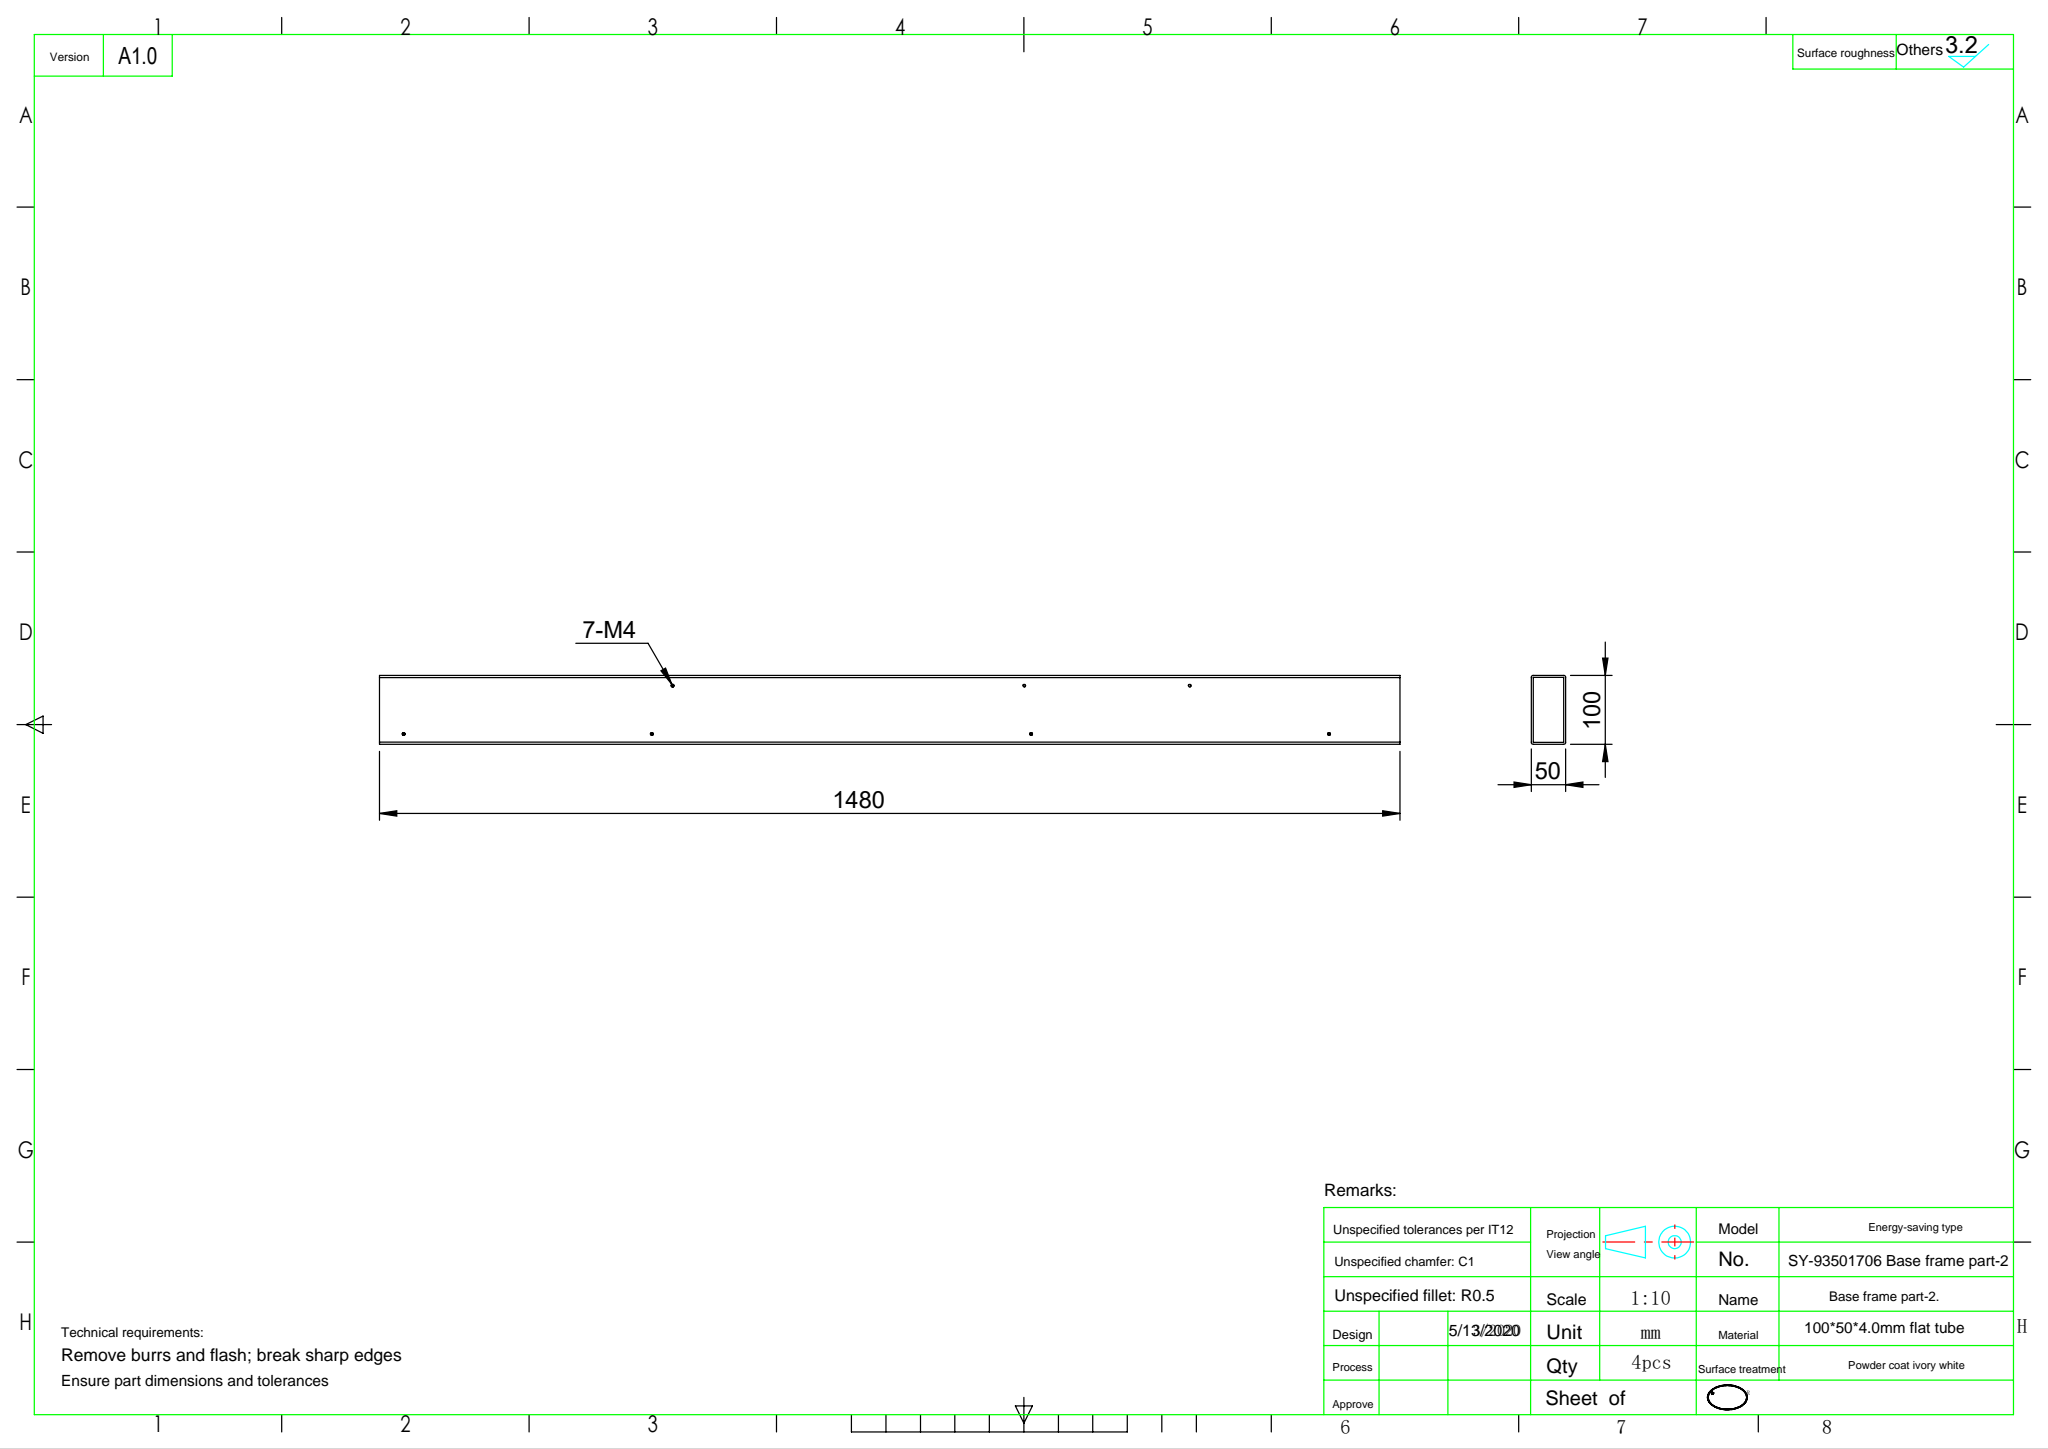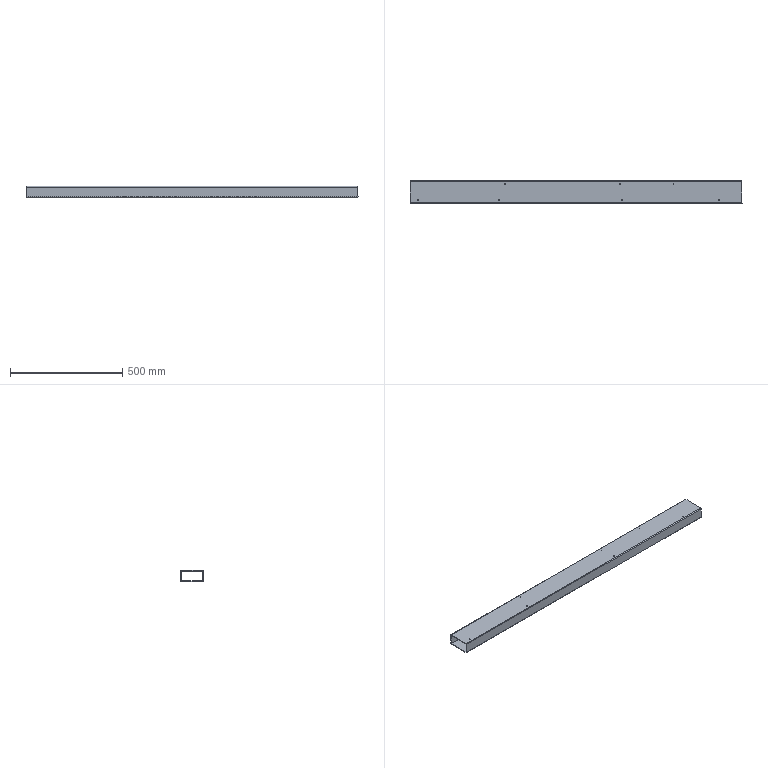Part | SolidWorks | features HoleWzd 3, BaseBody 1, ICE 1, MoveFace 1 | 1 solid | 42 faces | box 1480 x 100 x 50 mm | volume 1265578 mm3 | cylinder 22 | cone 10 | plane 10 | commonest cylinder face diameters 3.3 x14 0.4 x4 6.4 x4